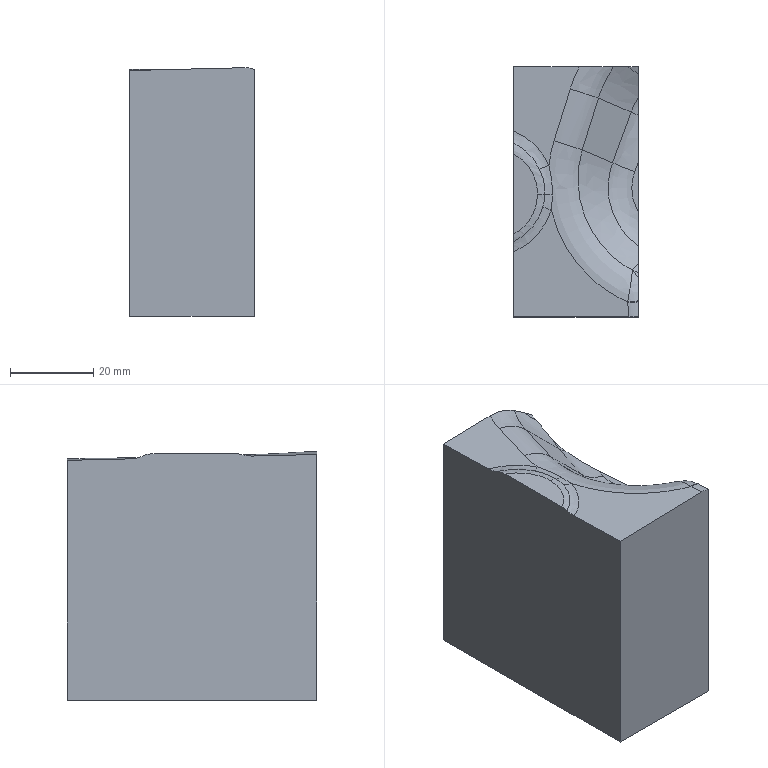Part | NX | features solid 2 | 1 solid | 30 faces | box 30.002 x 60 x 59.693 mm | volume 100958 mm3 | spline 25 | plane 5